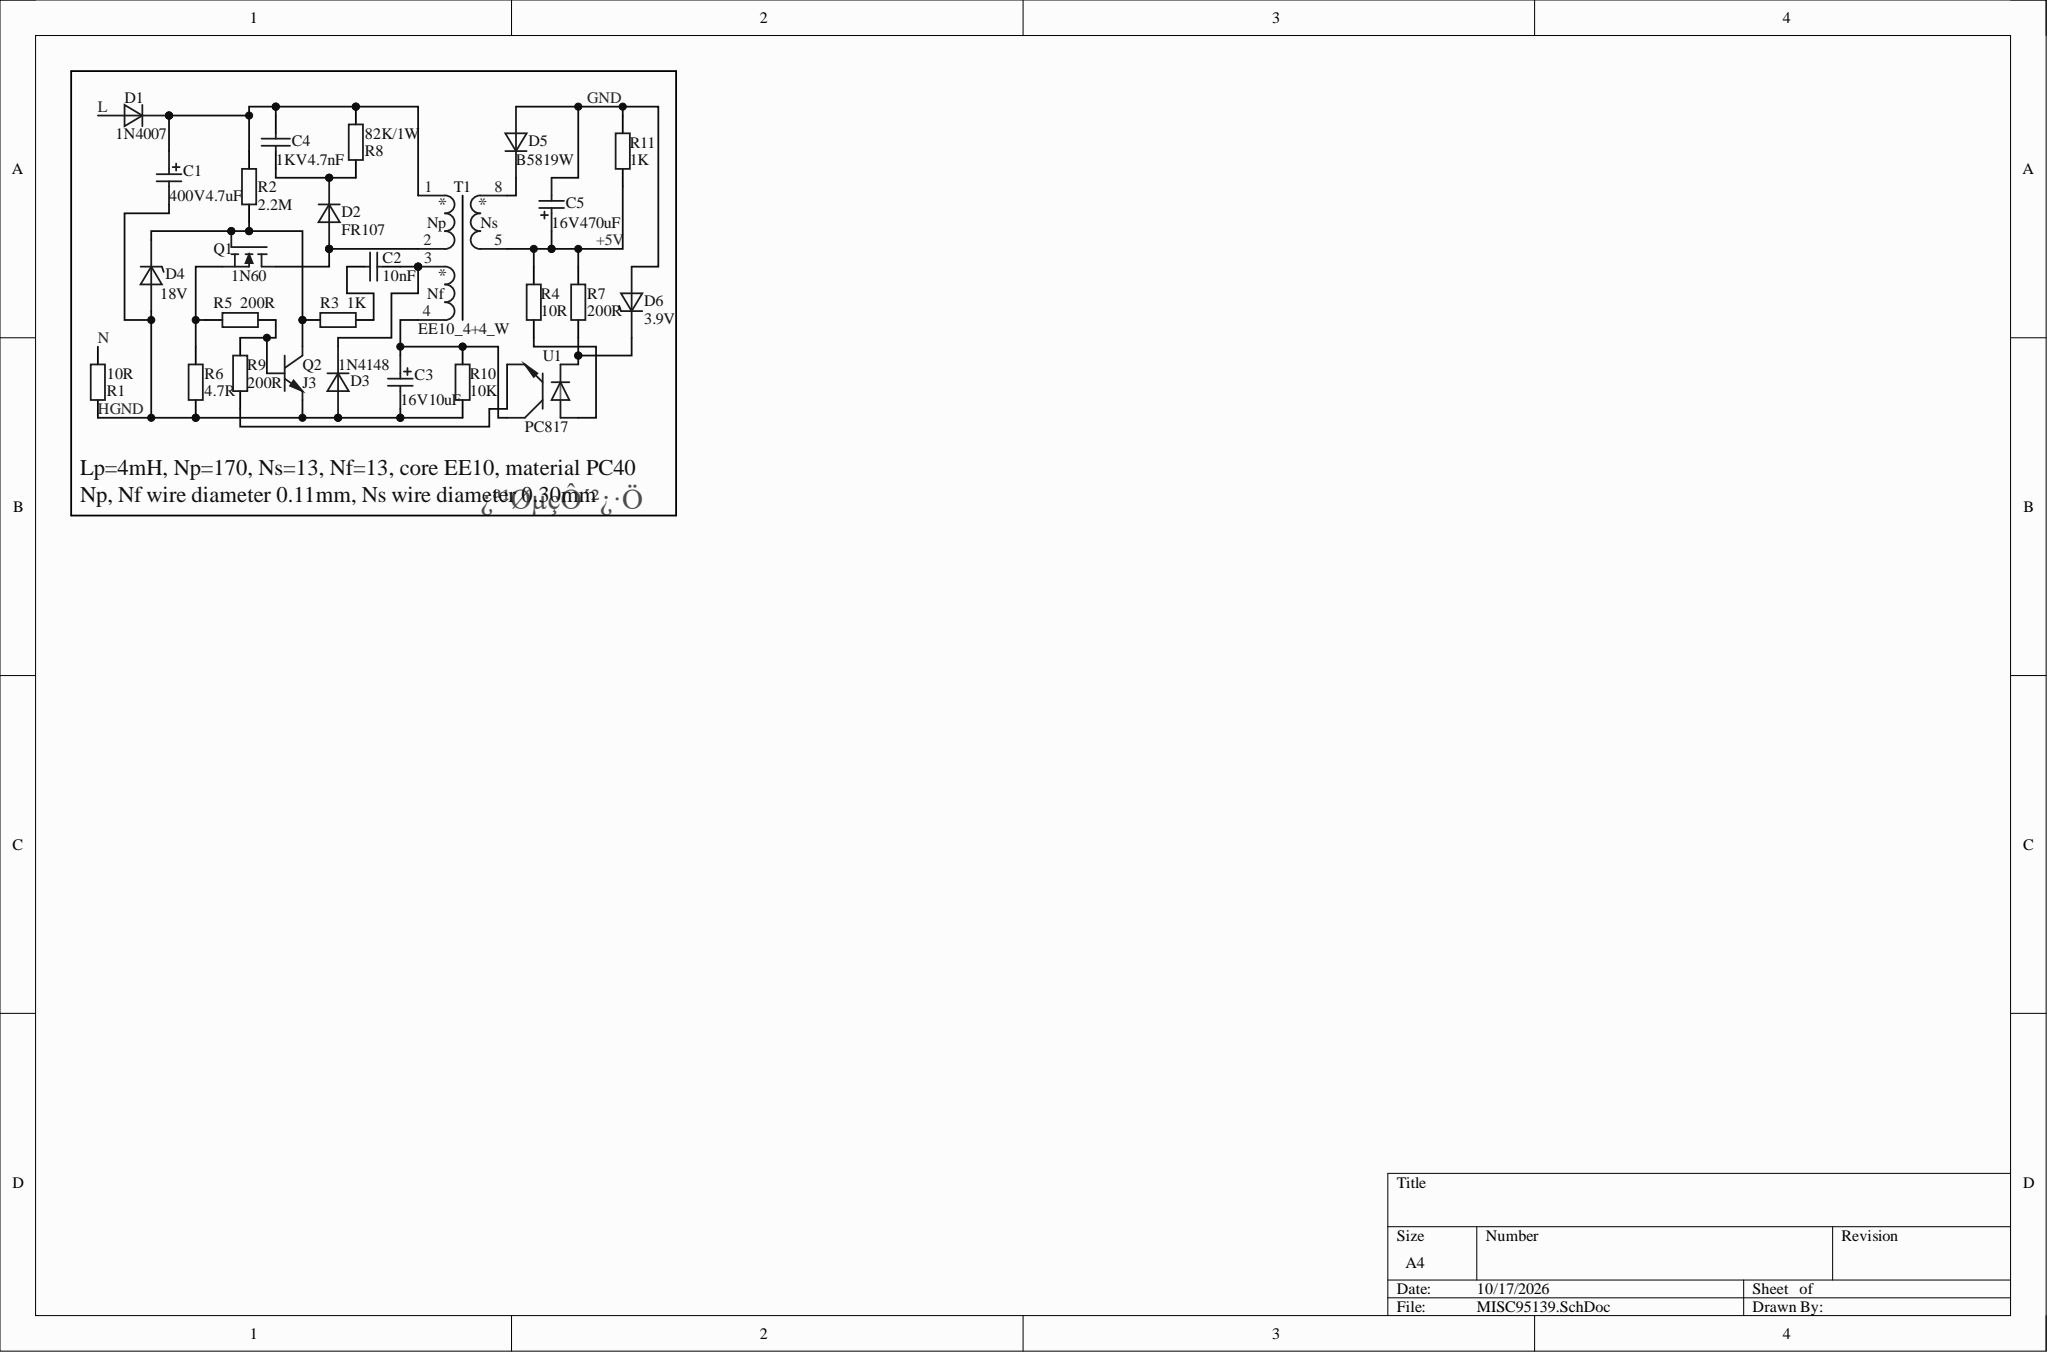Circuit board | Altium Designer | 26 parts | 16 nets
Bill of materials:
Comment,Description,Designator,Footprint,LibRef,Quantity
"400V4.7uF","","C1","cap-8*14mm","Cap Pol","1"
"10nF","Capacitor","C2","0805_Cap","Cap","1"
"16V10uF","","C3","0805_Cap","Cap Pol","1"
"1KV4.7nF","Capacitor","C4","CAP_5mm","Cap","1"
"16V470uF","","C5","cap-8*14mm","Cap Pol","1"
"1N4007","","D1","SOD-123","Diode","1"
"FR107","","D2","SOD-123","Diode","1"
"1N4148","","D3","SOD-123","Diode","1"
"18V","","D4","SOD-123","DZener","1"
"B5819W","","D5","SOD-123","Diode","1"
"3.9V","","D6","SOD-123","DZener","1"
"1N60","600V 20A N-Channel MOSFET","Q1","TO-126","FQPF20N60C","1"
"J3","SMD 9013 NPN-Transistor Vceo=25V,Icm=0.5A","Q2","SOT23","J3","1"
"10R","Resistor","R1, R4","0805_Res","Res2","2"
"2.2M","Resistor","R2","0805_Res","Res2","1"
"1K","Resistor","R3, R11","0805_Res","Res2","2"
"200R","Resistor","R5, R7, R9","0805_Res","Res2","3"
"4.7R","Resistor","R6","0805_Res","Res2","1"
"82K/1W","Resistor","R8","1W_Res_L","Res2","1"
"10K","Resistor","R10","0805_Res","Res2","1"
"EE10_4+4_W","","T1","EE10_4+4_W","Flyback transformer-1","1"
"PC817","Device Specification For PhotoCoupler","U1","SOP4-PC817","PC817","1"
Netlist (Protel format):
[
C1
cap-8*14mm
400V4.7uF



]
[
C2
0805_Cap
10nF



]
[
C3
0805_Cap
16V10uF



]
[
C4
CAP_5mm
1KV4.7nF



]
[
C5
cap-8*14mm
16V470uF



]
[
D1
SOD-123
1N4007



]
[
D2
SOD-123
FR107



]
[
D3
SOD-123
1N4148



]
[
D4
SOD-123
18V



]
[
D5
SOD-123
B5819W



]
[
D6
SOD-123
3.9V



]
[
Q1
TO-126
1N60



]
[
Q2
SOT23
J3



]
[
R1
0805_Res
10R



]
[
R2
0805_Res
2.2M



]
[
R3
0805_Res
1K



]
[
R4
0805_Res
10R



]
[
R5
0805_Res
200R



]
[
R6
0805_Res
4.7R



]
[
R7
0805_Res
200R



]
[
R8
1W_Res_L
82K/1W



]
[
R9
0805_Res
200R



]
[
R10
0805_Res
10K



]
[
R11
0805_Res
1K



]
[
T1
EE10_4+4_W
EE10_4+4_W



]
[
U1
SOP4-PC817
PC817



]
(
NetR9_1
R9-1
U1-3
)
(
NetR4_2
R4-2
U1-1
)
(
NetQ2_1
Q2-1
R5-1
R9-2
)
(
NetQ1_3
Q1-3
R5-2
R6-1
)
(
NetD6_2
D6-2
R7-1
U1-2
)
(
NetD5_2
D5-2
T1-8
)
(
NetD4_2
D4-2
Q1-1
Q2-3
R2-2
R3-1
)
(
NetD2_1
D2-1
Q1-2
T1-2
)
(
NetC4_2
C4-2
D2-2
R8-2
)
(
NetC3_1
C3-1
R10-1
T1-4
U1-4
)
(
NetC2_2
C2-2
R3-2
)
(
NetC2_1
C2-1
D3-2
T1-3
)
(
NetC1_1
C1-1
C4-1
D1-2
R2-1
R8-1
T1-1
)
(
HGND
C1-2
C3-2
D3-1
D4-1
Q2-2
R1-2
R6-2
R10-2
)
(
GND
C5-2
D5-1
D6-1
R11-1
)
(
+5V
C5-1
R4-1
R7-2
R11-2
T1-5
)